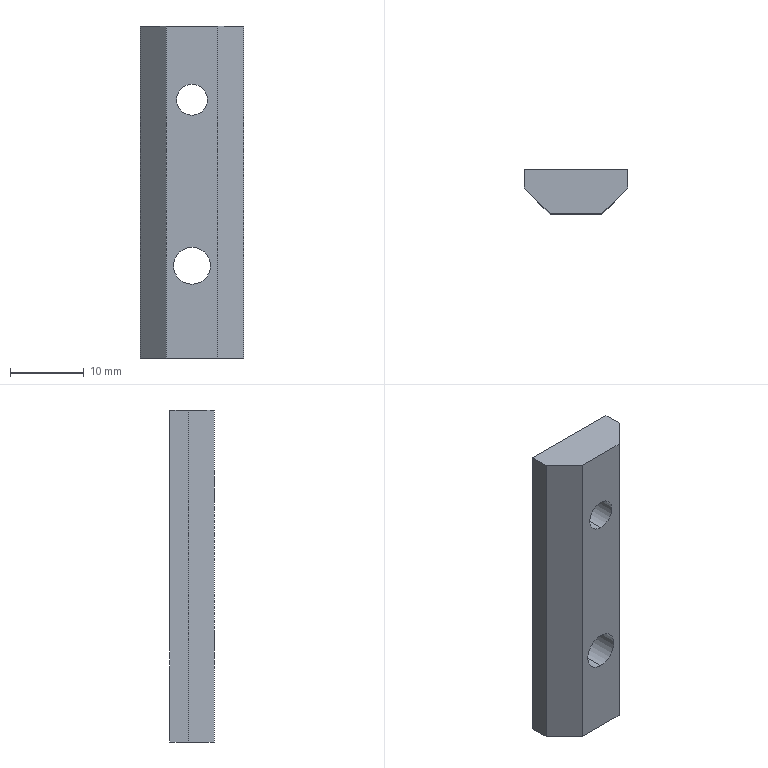Part | SolidWorks | features BaseBody 1 | 1 solid | 12 faces | box 14 x 6 x 45 mm | volume 3028 mm3 | plane 8 | cylinder 4 | commonest cylinder face diameters 4.2 x2 5 x2
STEP:
#1=CARTESIAN_POINT('',(0.,-6.,-2.1));
#2=VERTEX_POINT('',#1);
#3=CARTESIAN_POINT('',(0.,-6.,2.1));
#4=VERTEX_POINT('',#3);
#5=CARTESIAN_POINT('',(0.,-6.,0.));
#6=DIRECTION('',(0.,1.,0.));
#7=DIRECTION('',(-1.,0.,0.));
#8=AXIS2_PLACEMENT_3D('',#5,#6,#7);
#9=CIRCLE('',#8,2.1);
#10=EDGE_CURVE('',#2,#4,#9,.T.);
#11=ORIENTED_EDGE('',*,*,#10,.F.);
#12=CARTESIAN_POINT('',(0.,0.,-2.1));
#13=VERTEX_POINT('',#12);
#14=CARTESIAN_POINT('',(0.,0.,-2.1));
#15=DIRECTION('',(0.,1.,0.));
#16=VECTOR('',#15,1000.);
#17=LINE('',#14,#16);
#18=EDGE_CURVE('',#2,#13,#17,.T.);
#19=ORIENTED_EDGE('',*,*,#18,.T.);
#20=CARTESIAN_POINT('',(0.,0.,2.1));
#21=VERTEX_POINT('',#20);
#22=CARTESIAN_POINT('',(0.,0.,0.));
#23=DIRECTION('',(0.,1.,0.));
#24=DIRECTION('',(0.,0.,1.));
#25=AXIS2_PLACEMENT_3D('',#22,#23,#24);
#26=CIRCLE('',#25,2.1);
#27=EDGE_CURVE('',#13,#21,#26,.T.);
#28=ORIENTED_EDGE('',*,*,#27,.T.);
#29=CARTESIAN_POINT('',(0.,0.,2.1));
#30=DIRECTION('',(0.,1.,0.));
#31=VECTOR('',#30,1000.);
#32=LINE('',#29,#31);
#33=EDGE_CURVE('',#4,#21,#32,.T.);
#34=ORIENTED_EDGE('',*,*,#33,.F.);
#35=EDGE_LOOP('',(#11,#19,#28,#34));
#36=FACE_OUTER_BOUND('',#35,.T.);
#37=CARTESIAN_POINT('',(0.,0.,0.));
#38=DIRECTION('',(0.,1.,0.));
#39=DIRECTION('',(0.,0.,1.));
#40=AXIS2_PLACEMENT_3D('',#37,#38,#39);
#41=CYLINDRICAL_SURFACE('',#40,2.1);
#42=ADVANCED_FACE('',(#36),#41,.F.);
#43=CARTESIAN_POINT('',(0.,-6.,-25.));
#44=VERTEX_POINT('',#43);
#45=CARTESIAN_POINT('',(0.,-6.,-20.));
#46=VERTEX_POINT('',#45);
#47=CARTESIAN_POINT('',(0.,-6.,-22.5));
#48=DIRECTION('',(0.,1.,0.));
#49=DIRECTION('',(-1.,0.,0.));
#50=AXIS2_PLACEMENT_3D('',#47,#48,#49);
#51=CIRCLE('',#50,2.5);
#52=EDGE_CURVE('',#44,#46,#51,.T.);
#53=ORIENTED_EDGE('',*,*,#52,.F.);
#54=CARTESIAN_POINT('',(0.,0.,-25.));
#55=VERTEX_POINT('',#54);
#56=CARTESIAN_POINT('',(0.,0.,-25.));
#57=DIRECTION('',(0.,1.,0.));
#58=VECTOR('',#57,1000.);
#59=LINE('',#56,#58);
#60=EDGE_CURVE('',#44,#55,#59,.T.);
#61=ORIENTED_EDGE('',*,*,#60,.T.);
#62=CARTESIAN_POINT('',(0.,0.,-20.));
#63=VERTEX_POINT('',#62);
#64=CARTESIAN_POINT('',(0.,0.,-22.5));
#65=DIRECTION('',(0.,1.,0.));
#66=DIRECTION('',(0.,0.,1.));
#67=AXIS2_PLACEMENT_3D('',#64,#65,#66);
#68=CIRCLE('',#67,2.5);
#69=EDGE_CURVE('',#55,#63,#68,.T.);
#70=ORIENTED_EDGE('',*,*,#69,.T.);
#71=CARTESIAN_POINT('',(0.,0.,-20.));
#72=DIRECTION('',(0.,1.,0.));
#73=VECTOR('',#72,1000.);
#74=LINE('',#71,#73);
#75=EDGE_CURVE('',#46,#63,#74,.T.);
#76=ORIENTED_EDGE('',*,*,#75,.F.);
#77=EDGE_LOOP('',(#53,#61,#70,#76));
#78=FACE_OUTER_BOUND('',#77,.T.);
#79=CARTESIAN_POINT('',(0.,0.,-22.5));
#80=DIRECTION('',(0.,1.,0.));
#81=DIRECTION('',(0.,0.,1.));
#82=AXIS2_PLACEMENT_3D('',#79,#80,#81);
#83=CYLINDRICAL_SURFACE('',#82,2.5);
#84=ADVANCED_FACE('',(#78),#83,.F.);
#85=CARTESIAN_POINT('',(3.5,-6.,10.));
#86=VERTEX_POINT('',#85);
#87=CARTESIAN_POINT('',(-3.5,-6.,10.));
#88=VERTEX_POINT('',#87);
#89=CARTESIAN_POINT('',(-7.,-6.,10.));
#90=DIRECTION('',(-1.,0.,0.));
#91=VECTOR('',#90,1000.);
#92=LINE('',#89,#91);
#93=EDGE_CURVE('',#86,#88,#92,.T.);
#94=ORIENTED_EDGE('',*,*,#93,.F.);
#95=CARTESIAN_POINT('',(7.,-2.5,10.));
#96=VERTEX_POINT('',#95);
#97=CARTESIAN_POINT('',(7.,-2.5,10.));
#98=DIRECTION('',(-0.7071,-0.7071,0.));
#99=VECTOR('',#98,1000.);
#100=LINE('',#97,#99);
#101=EDGE_CURVE('',#96,#86,#100,.T.);
#102=ORIENTED_EDGE('',*,*,#101,.F.);
#103=CARTESIAN_POINT('',(7.,0.,10.));
#104=VERTEX_POINT('',#103);
#105=CARTESIAN_POINT('',(7.,-6.,10.));
#106=DIRECTION('',(0.,1.,0.));
#107=VECTOR('',#106,1000.);
#108=LINE('',#105,#107);
#109=EDGE_CURVE('',#96,#104,#108,.T.);
#110=ORIENTED_EDGE('',*,*,#109,.T.);
#111=CARTESIAN_POINT('',(-7.,0.,10.));
#112=VERTEX_POINT('',#111);
#113=CARTESIAN_POINT('',(-7.,0.,10.));
#114=DIRECTION('',(-1.,0.,0.));
#115=VECTOR('',#114,1000.);
#116=LINE('',#113,#115);
#117=EDGE_CURVE('',#104,#112,#116,.T.);
#118=ORIENTED_EDGE('',*,*,#117,.T.);
#119=CARTESIAN_POINT('',(-7.,-2.5,10.));
#120=VERTEX_POINT('',#119);
#121=CARTESIAN_POINT('',(-7.,-6.,10.));
#122=DIRECTION('',(0.,1.,0.));
#123=VECTOR('',#122,1000.);
#124=LINE('',#121,#123);
#125=EDGE_CURVE('',#120,#112,#124,.T.);
#126=ORIENTED_EDGE('',*,*,#125,.F.);
#127=CARTESIAN_POINT('',(-3.5,-6.,10.));
#128=DIRECTION('',(-0.7071,0.7071,0.));
#129=VECTOR('',#128,1000.);
#130=LINE('',#127,#129);
#131=EDGE_CURVE('',#88,#120,#130,.T.);
#132=ORIENTED_EDGE('',*,*,#131,.F.);
#133=EDGE_LOOP('',(#94,#102,#110,#118,#126,#132));
#134=FACE_OUTER_BOUND('',#133,.T.);
#135=CARTESIAN_POINT('',(-7.,-6.,10.));
#136=DIRECTION('',(0.,0.,-1.));
#137=DIRECTION('',(0.,-1.,0.));
#138=AXIS2_PLACEMENT_3D('',#135,#136,#137);
#139=PLANE('',#138);
#140=ADVANCED_FACE('',(#134),#139,.F.);
#141=CARTESIAN_POINT('',(-7.,0.,-35.));
#142=VERTEX_POINT('',#141);
#143=CARTESIAN_POINT('',(-7.,-2.5,-35.));
#144=VERTEX_POINT('',#143);
#145=CARTESIAN_POINT('',(-7.,-2.5,-35.));
#146=DIRECTION('',(0.,-1.,0.));
#147=VECTOR('',#146,1000.);
#148=LINE('',#145,#147);
#149=EDGE_CURVE('',#142,#144,#148,.T.);
#150=ORIENTED_EDGE('',*,*,#149,.F.);
#151=CARTESIAN_POINT('',(7.,0.,-35.));
#152=VERTEX_POINT('',#151);
#153=CARTESIAN_POINT('',(-7.,0.,-35.));
#154=DIRECTION('',(-1.,0.,0.));
#155=VECTOR('',#154,1000.);
#156=LINE('',#153,#155);
#157=EDGE_CURVE('',#152,#142,#156,.T.);
#158=ORIENTED_EDGE('',*,*,#157,.F.);
#159=CARTESIAN_POINT('',(7.,-2.5,-35.));
#160=VERTEX_POINT('',#159);
#161=CARTESIAN_POINT('',(7.,0.,-35.));
#162=DIRECTION('',(0.,1.,0.));
#163=VECTOR('',#162,1000.);
#164=LINE('',#161,#163);
#165=EDGE_CURVE('',#160,#152,#164,.T.);
#166=ORIENTED_EDGE('',*,*,#165,.F.);
#167=CARTESIAN_POINT('',(3.5,-6.,-35.));
#168=VERTEX_POINT('',#167);
#169=CARTESIAN_POINT('',(7.,-2.5,-35.));
#170=DIRECTION('',(0.7071,0.7071,0.));
#171=VECTOR('',#170,1000.);
#172=LINE('',#169,#171);
#173=EDGE_CURVE('',#168,#160,#172,.T.);
#174=ORIENTED_EDGE('',*,*,#173,.F.);
#175=CARTESIAN_POINT('',(-3.5,-6.,-35.));
#176=VERTEX_POINT('',#175);
#177=CARTESIAN_POINT('',(3.5,-6.,-35.));
#178=DIRECTION('',(1.,0.,0.));
#179=VECTOR('',#178,1000.);
#180=LINE('',#177,#179);
#181=EDGE_CURVE('',#176,#168,#180,.T.);
#182=ORIENTED_EDGE('',*,*,#181,.F.);
#183=CARTESIAN_POINT('',(-3.5,-6.,-35.));
#184=DIRECTION('',(0.7071,-0.7071,0.));
#185=VECTOR('',#184,1000.);
#186=LINE('',#183,#185);
#187=EDGE_CURVE('',#144,#176,#186,.T.);
#188=ORIENTED_EDGE('',*,*,#187,.F.);
#189=EDGE_LOOP('',(#150,#158,#166,#174,#182,#188));
#190=FACE_OUTER_BOUND('',#189,.T.);
#191=CARTESIAN_POINT('',(0.,0.,-35.));
#192=DIRECTION('',(0.,0.,-1.));
#193=DIRECTION('',(0.,-1.,0.));
#194=AXIS2_PLACEMENT_3D('',#191,#192,#193);
#195=PLANE('',#194);
#196=ADVANCED_FACE('',(#190),#195,.T.);
#197=CARTESIAN_POINT('',(7.,0.,35.));
#198=DIRECTION('',(0.,0.,-1.));
#199=VECTOR('',#198,1000.);
#200=LINE('',#197,#199);
#201=EDGE_CURVE('',#104,#152,#200,.T.);
#202=ORIENTED_EDGE('',*,*,#201,.F.);
#203=ORIENTED_EDGE('',*,*,#109,.F.);
#204=CARTESIAN_POINT('',(7.,-2.5,35.));
#205=DIRECTION('',(0.,0.,-1.));
#206=VECTOR('',#205,1000.);
#207=LINE('',#204,#206);
#208=EDGE_CURVE('',#96,#160,#207,.T.);
#209=ORIENTED_EDGE('',*,*,#208,.T.);
#210=ORIENTED_EDGE('',*,*,#165,.T.);
#211=EDGE_LOOP('',(#202,#203,#209,#210));
#212=FACE_OUTER_BOUND('',#211,.T.);
#213=CARTESIAN_POINT('',(7.,0.,35.));
#214=DIRECTION('',(-1.,0.,0.));
#215=DIRECTION('',(0.,0.,1.));
#216=AXIS2_PLACEMENT_3D('',#213,#214,#215);
#217=PLANE('',#216);
#218=ADVANCED_FACE('',(#212),#217,.F.);
#219=ORIENTED_EDGE('',*,*,#208,.F.);
#220=ORIENTED_EDGE('',*,*,#101,.T.);
#221=CARTESIAN_POINT('',(3.5,-6.,35.));
#222=DIRECTION('',(0.,0.,-1.));
#223=VECTOR('',#222,1000.);
#224=LINE('',#221,#223);
#225=EDGE_CURVE('',#86,#168,#224,.T.);
#226=ORIENTED_EDGE('',*,*,#225,.T.);
#227=ORIENTED_EDGE('',*,*,#173,.T.);
#228=EDGE_LOOP('',(#219,#220,#226,#227));
#229=FACE_OUTER_BOUND('',#228,.T.);
#230=CARTESIAN_POINT('',(7.,-2.5,35.));
#231=DIRECTION('',(-0.7071,0.7071,0.));
#232=DIRECTION('',(0.,0.,1.));
#233=AXIS2_PLACEMENT_3D('',#230,#231,#232);
#234=PLANE('',#233);
#235=ADVANCED_FACE('',(#229),#234,.F.);
#236=CARTESIAN_POINT('',(0.,-6.,-22.5));
#237=DIRECTION('',(0.,1.,0.));
#238=DIRECTION('',(-1.,0.,0.));
#239=AXIS2_PLACEMENT_3D('',#236,#237,#238);
#240=CIRCLE('',#239,2.5);
#241=EDGE_CURVE('',#46,#44,#240,.T.);
#242=ORIENTED_EDGE('',*,*,#241,.T.);
#243=ORIENTED_EDGE('',*,*,#52,.T.);
#244=EDGE_LOOP('',(#242,#243));
#245=FACE_BOUND('',#244,.T.);
#246=CARTESIAN_POINT('',(0.,-6.,0.));
#247=DIRECTION('',(0.,1.,0.));
#248=DIRECTION('',(-1.,0.,0.));
#249=AXIS2_PLACEMENT_3D('',#246,#247,#248);
#250=CIRCLE('',#249,2.1);
#251=EDGE_CURVE('',#4,#2,#250,.T.);
#252=ORIENTED_EDGE('',*,*,#251,.T.);
#253=ORIENTED_EDGE('',*,*,#10,.T.);
#254=EDGE_LOOP('',(#252,#253));
#255=FACE_BOUND('',#254,.T.);
#256=ORIENTED_EDGE('',*,*,#225,.F.);
#257=ORIENTED_EDGE('',*,*,#93,.T.);
#258=CARTESIAN_POINT('',(-3.5,-6.,35.));
#259=DIRECTION('',(0.,0.,-1.));
#260=VECTOR('',#259,1000.);
#261=LINE('',#258,#260);
#262=EDGE_CURVE('',#88,#176,#261,.T.);
#263=ORIENTED_EDGE('',*,*,#262,.T.);
#264=ORIENTED_EDGE('',*,*,#181,.T.);
#265=EDGE_LOOP('',(#256,#257,#263,#264));
#266=FACE_OUTER_BOUND('',#265,.T.);
#267=CARTESIAN_POINT('',(3.5,-6.,35.));
#268=DIRECTION('',(0.,1.,0.));
#269=DIRECTION('',(1.,0.,0.));
#270=AXIS2_PLACEMENT_3D('',#267,#268,#269);
#271=PLANE('',#270);
#272=ADVANCED_FACE('',(#245,#255,#266),#271,.F.);
#273=ORIENTED_EDGE('',*,*,#262,.F.);
#274=ORIENTED_EDGE('',*,*,#131,.T.);
#275=CARTESIAN_POINT('',(-7.,-2.5,35.));
#276=DIRECTION('',(0.,0.,-1.));
#277=VECTOR('',#276,1000.);
#278=LINE('',#275,#277);
#279=EDGE_CURVE('',#120,#144,#278,.T.);
#280=ORIENTED_EDGE('',*,*,#279,.T.);
#281=ORIENTED_EDGE('',*,*,#187,.T.);
#282=EDGE_LOOP('',(#273,#274,#280,#281));
#283=FACE_OUTER_BOUND('',#282,.T.);
#284=CARTESIAN_POINT('',(-3.5,-6.,35.));
#285=DIRECTION('',(0.7071,0.7071,0.));
#286=DIRECTION('',(0.,0.,-1.));
#287=AXIS2_PLACEMENT_3D('',#284,#285,#286);
#288=PLANE('',#287);
#289=ADVANCED_FACE('',(#283),#288,.F.);
#290=ORIENTED_EDGE('',*,*,#279,.F.);
#291=ORIENTED_EDGE('',*,*,#125,.T.);
#292=CARTESIAN_POINT('',(-7.,0.,35.));
#293=DIRECTION('',(0.,0.,-1.));
#294=VECTOR('',#293,1000.);
#295=LINE('',#292,#294);
#296=EDGE_CURVE('',#112,#142,#295,.T.);
#297=ORIENTED_EDGE('',*,*,#296,.T.);
#298=ORIENTED_EDGE('',*,*,#149,.T.);
#299=EDGE_LOOP('',(#290,#291,#297,#298));
#300=FACE_OUTER_BOUND('',#299,.T.);
#301=CARTESIAN_POINT('',(-7.,-2.5,35.));
#302=DIRECTION('',(1.,0.,0.));
#303=DIRECTION('',(0.,1.,0.));
#304=AXIS2_PLACEMENT_3D('',#301,#302,#303);
#305=PLANE('',#304);
#306=ADVANCED_FACE('',(#300),#305,.F.);
#307=CARTESIAN_POINT('',(0.,0.,-22.5));
#308=DIRECTION('',(0.,1.,0.));
#309=DIRECTION('',(0.,0.,1.));
#310=AXIS2_PLACEMENT_3D('',#307,#308,#309);
#311=CIRCLE('',#310,2.5);
#312=EDGE_CURVE('',#63,#55,#311,.T.);
#313=ORIENTED_EDGE('',*,*,#312,.F.);
#314=ORIENTED_EDGE('',*,*,#69,.F.);
#315=EDGE_LOOP('',(#313,#314));
#316=FACE_BOUND('',#315,.T.);
#317=CARTESIAN_POINT('',(0.,0.,0.));
#318=DIRECTION('',(0.,1.,0.));
#319=DIRECTION('',(0.,0.,1.));
#320=AXIS2_PLACEMENT_3D('',#317,#318,#319);
#321=CIRCLE('',#320,2.1);
#322=EDGE_CURVE('',#21,#13,#321,.T.);
#323=ORIENTED_EDGE('',*,*,#322,.F.);
#324=ORIENTED_EDGE('',*,*,#27,.F.);
#325=EDGE_LOOP('',(#323,#324));
#326=FACE_BOUND('',#325,.T.);
#327=ORIENTED_EDGE('',*,*,#296,.F.);
#328=ORIENTED_EDGE('',*,*,#117,.F.);
#329=ORIENTED_EDGE('',*,*,#201,.T.);
#330=ORIENTED_EDGE('',*,*,#157,.T.);
#331=EDGE_LOOP('',(#327,#328,#329,#330));
#332=FACE_OUTER_BOUND('',#331,.T.);
#333=CARTESIAN_POINT('',(-7.,0.,35.));
#334=DIRECTION('',(0.,-1.,0.));
#335=DIRECTION('',(0.,0.,-1.));
#336=AXIS2_PLACEMENT_3D('',#333,#334,#335);
#337=PLANE('',#336);
#338=ADVANCED_FACE('',(#316,#326,#332),#337,.F.);
#339=ORIENTED_EDGE('',*,*,#60,.F.);
#340=ORIENTED_EDGE('',*,*,#241,.F.);
#341=ORIENTED_EDGE('',*,*,#75,.T.);
#342=ORIENTED_EDGE('',*,*,#312,.T.);
#343=EDGE_LOOP('',(#339,#340,#341,#342));
#344=FACE_OUTER_BOUND('',#343,.T.);
#345=CARTESIAN_POINT('',(0.,0.,-22.5));
#346=DIRECTION('',(0.,1.,0.));
#347=DIRECTION('',(0.,0.,1.));
#348=AXIS2_PLACEMENT_3D('',#345,#346,#347);
#349=CYLINDRICAL_SURFACE('',#348,2.5);
#350=ADVANCED_FACE('',(#344),#349,.F.);
#351=ORIENTED_EDGE('',*,*,#18,.F.);
#352=ORIENTED_EDGE('',*,*,#251,.F.);
#353=ORIENTED_EDGE('',*,*,#33,.T.);
#354=ORIENTED_EDGE('',*,*,#322,.T.);
#355=EDGE_LOOP('',(#351,#352,#353,#354));
#356=FACE_OUTER_BOUND('',#355,.T.);
#357=CARTESIAN_POINT('',(0.,0.,0.));
#358=DIRECTION('',(0.,1.,0.));
#359=DIRECTION('',(0.,0.,1.));
#360=AXIS2_PLACEMENT_3D('',#357,#358,#359);
#361=CYLINDRICAL_SURFACE('',#360,2.1);
#362=ADVANCED_FACE('',(#356),#361,.F.);
#363=CLOSED_SHELL('',(#42,#84,#140,#196,#218,#235,#272,#289,#306,#338,#350,#362));
#364=MANIFOLD_SOLID_BREP('',#363);
#365=CARTESIAN_POINT('',(0.,0.,0.));
#366=DIRECTION('',(0.,0.,1.));
#367=DIRECTION('',(1.,0.,0.));
#368=AXIS2_PLACEMENT_3D('',#365,#366,#367);
#369=(LENGTH_UNIT()NAMED_UNIT(*)SI_UNIT(.MILLI.,.METRE.));
#370=UNCERTAINTY_MEASURE_WITH_UNIT(LENGTH_MEASURE(0.00001),#369,'','');
#371=(NAMED_UNIT(*)PLANE_ANGLE_UNIT()SI_UNIT($,.RADIAN.));
#372=(NAMED_UNIT(*)SI_UNIT($,.STERADIAN.)SOLID_ANGLE_UNIT());
#373=(GEOMETRIC_REPRESENTATION_CONTEXT(3)GLOBAL_UNCERTAINTY_ASSIGNED_CONTEXT((#370))GLOBAL_UNIT_ASSIGNED_CONTEXT((#369,#371,#372))REPRESENTATION_CONTEXT('',''));
#374=ADVANCED_BREP_SHAPE_REPRESENTATION('',(#364,#368),#373);